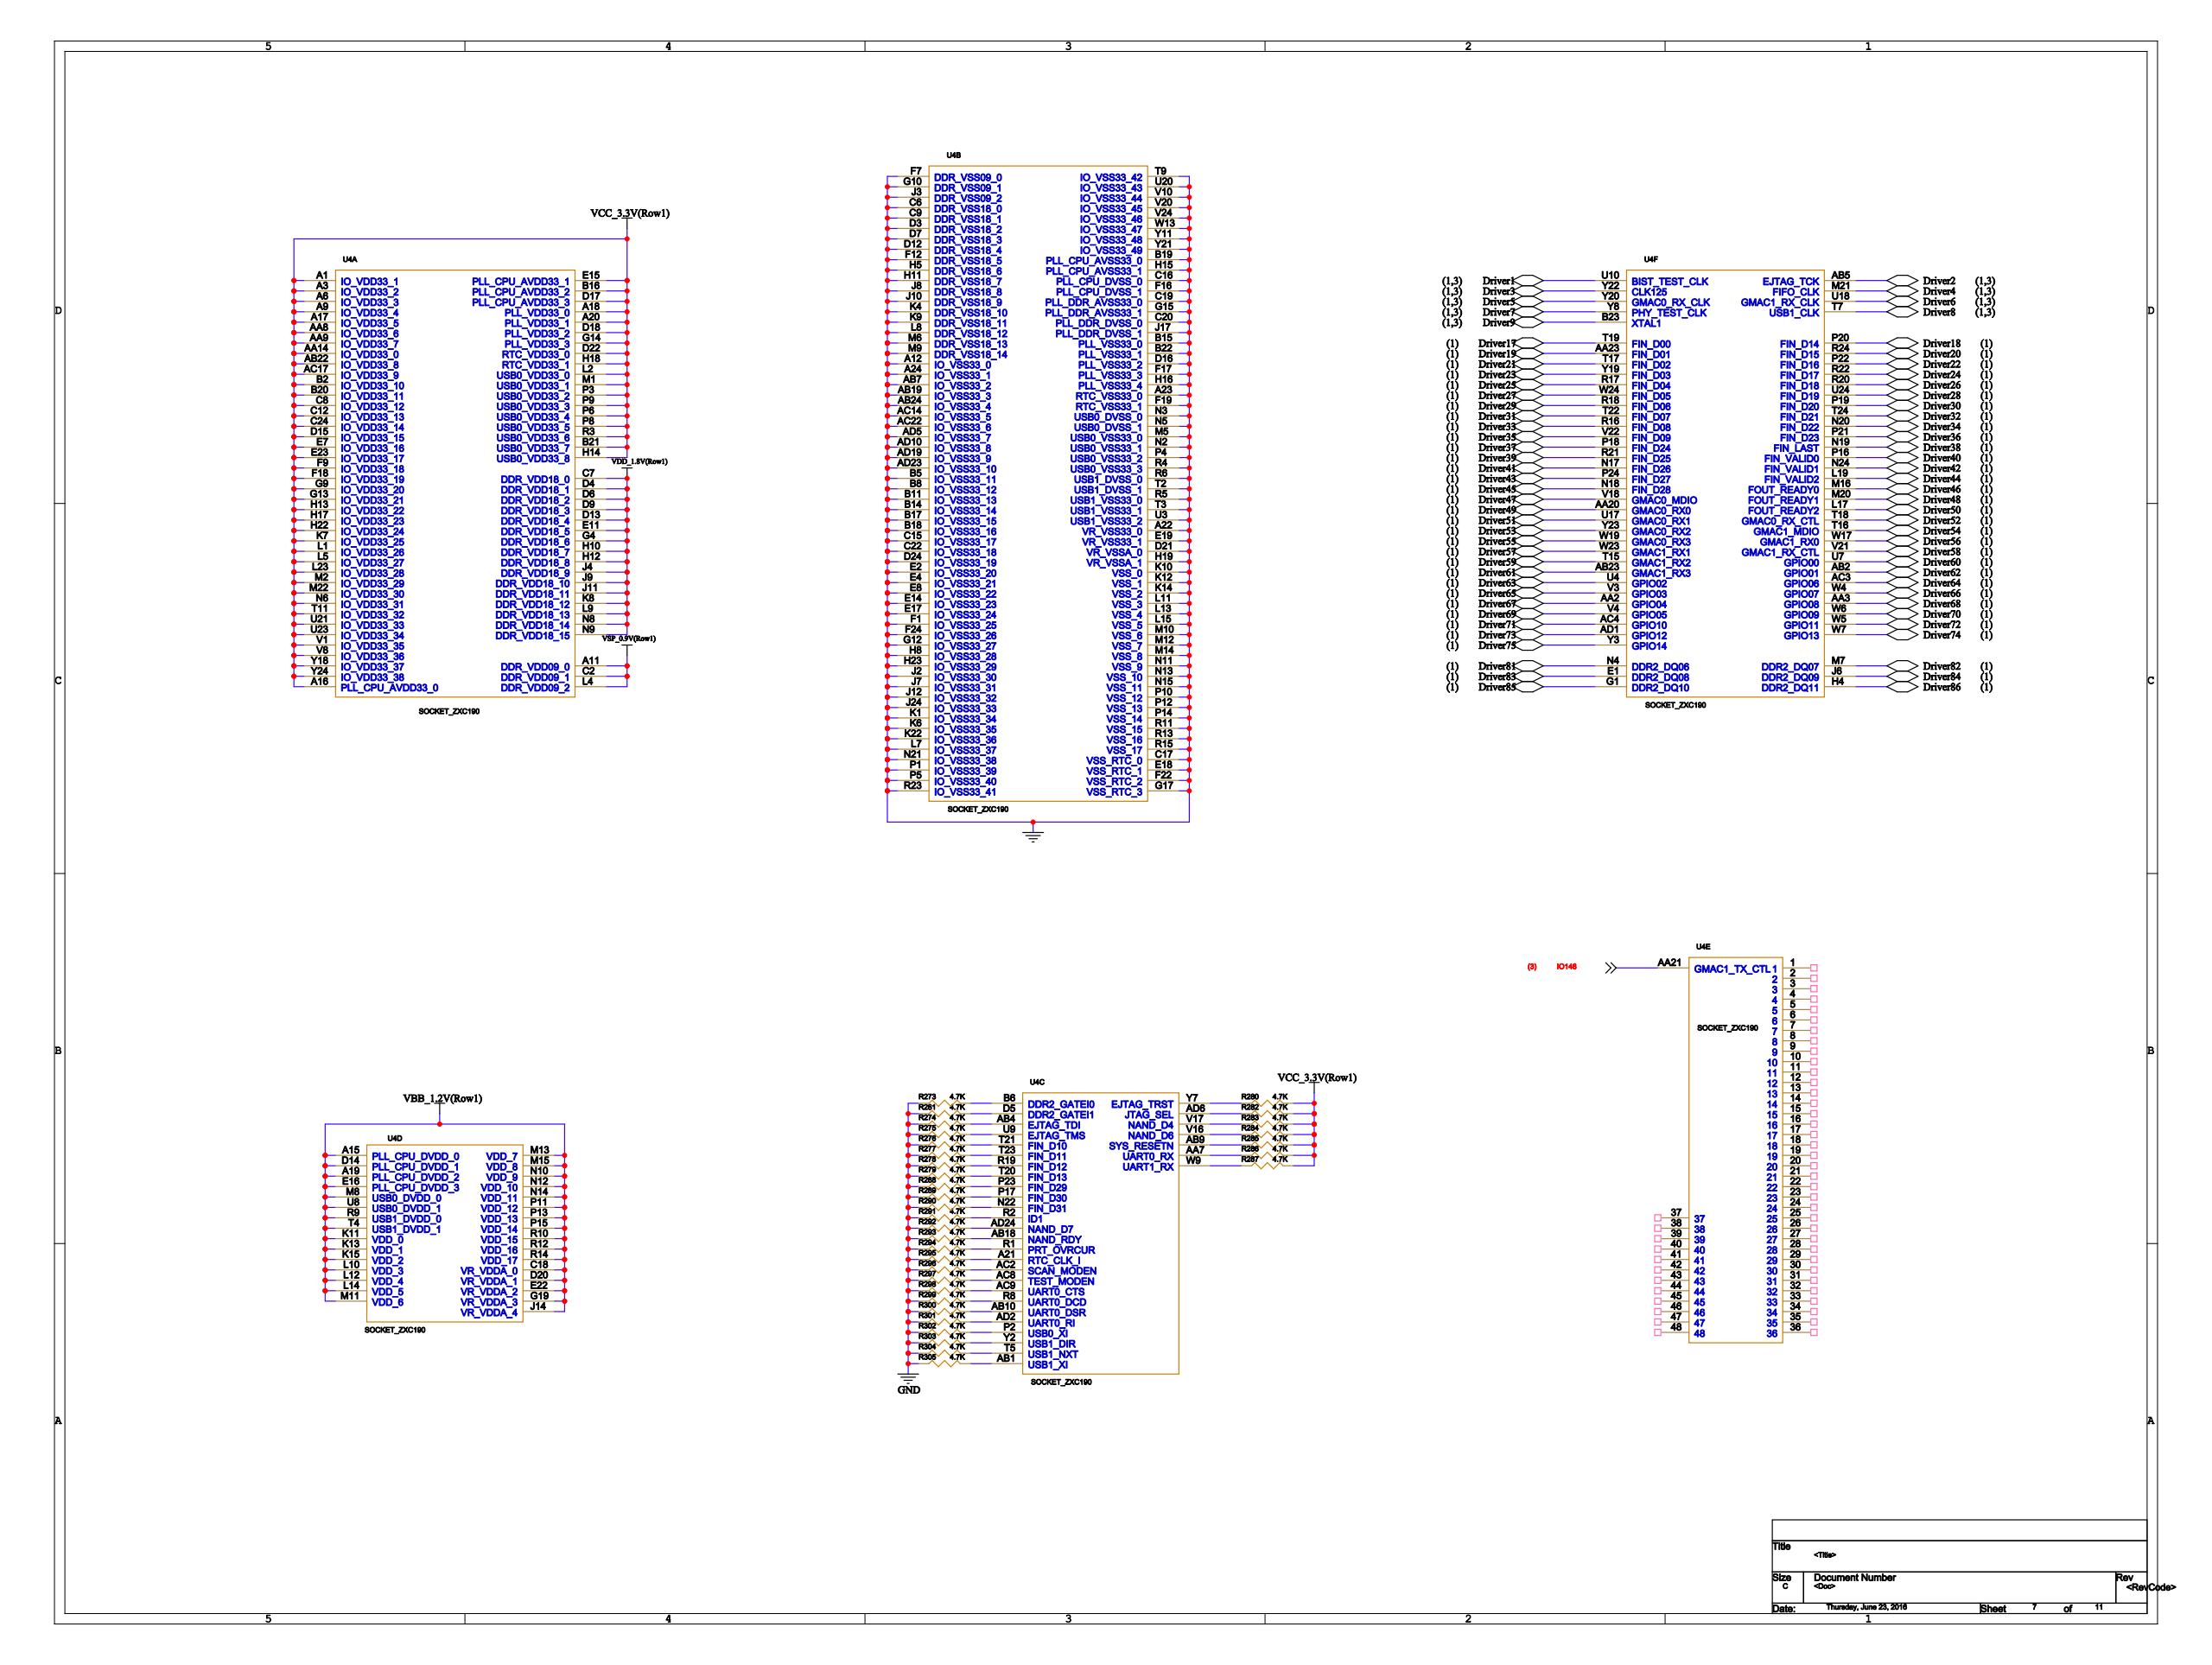Circuit board | Cadence Allegro | 531 parts | 624 nets | one sheet of the schematic
Parts on this sheet (reference | value | footprint):
R273 | 4.7K | R0805
R274 | 4.7K | R0805
R275 | 4.7K | R0805
R276 | 4.7K | R0805
R277 | 4.7K | R0805
R278 | 4.7K | R0805
R279 | 4.7K | R0805
R280 | 4.7K | R0805
R281 | 4.7K | R0805
R282 | 4.7K | R0805
R283 | 4.7K | R0805
R284 | 4.7K | R0805
R285 | 4.7K | R0805
R286 | 4.7K | R0805
R287 | 4.7K | R0805
R288 | 4.7K | R0805
R289 | 4.7K | R0805
R290 | 4.7K | R0805
R291 | 4.7K | R0805
R292 | 4.7K | R0805
R293 | 4.7K | R0805
R294 | 4.7K | R0805
R295 | 4.7K | R0805
R296 | 4.7K | R0805
R297 | 4.7K | R0805
R298 | 4.7K | R0805
R299 | 4.7K | R0805
R300 | 4.7K | R0805
R301 | 4.7K | R0805
R302 | 4.7K | R0805
R303 | 4.7K | R0805
R304 | 4.7K | R0805
R305 | 4.7K | R0805
U3 | SOCKET_ZXC190 | BGA-576
U4 | SOCKET_ZXC190 | BGA-576
U10 | SOCKET_ZXC190 | BGA-576
Nets of these parts (net: part-pin ...):
GND: R273-1 R274-1 R275-1 R276-1 R277-1 R278-1 R279-1 R281-1 R288-1 R289-1 R290-1 R291-1 R292-1 R293-1 R294-1 R295-1 R296-1 R297-1 R298-1 R299-1 R300-1 R301-1 R302-1 R303-1 R304-1 R305-1 U3-A12 U3-A22 U3-A23 U3-A24 U3-AB7 U3-AB19 U3-AB24 U3-AC14 U3-AC22 U3-AD5 U3-AD10 U3-AD19 U3-AD23 U3-B5 U3-B8 U3-B11 U3-B14 U3-B15 U3-B17 U3-B18 U3-B19 U3-B22 U3-C6 U3-C9 U3-C15 U3-C16 U3-C17 U3-C19 U3-C20 U3-C22 U3-D3 U3-D7 U3-D12 U3-D16 U3-D21 U3-D24 U3-E2 U3-E4 U3-E8 U3-E14 U3-E17 U3-E18 U3-E19 U3-F1 U3-F7 U3-F12 U3-F16 U3-F17 U3-F19 U3-F22 U3-F24 U3-G10 U3-G12 U3-G15 U3-G17 U3-H5 U3-H8 U3-H11 U3-H15 U3-H16 U3-H19 U3-H23 U3-J2 U3-J3 U3-J7 U3-J8 U3-J10 U3-J12 U3-J17 U3-J24 U3-K1 U3-K4 U3-K6 U3-K9 U3-K10 U3-K12 U3-K14 U3-K22 U3-L7 U3-L8 U3-L11 U3-L13 U3-L15 U3-M5 U3-M6 U3-M9 U3-M10 U3-M12 U3-M14 U3-N2 U3-N3 U3-N5 U3-N11 U3-N13 U3-N15 U3-N21 U3-P1 U3-P4 U3-P5 U3-P10 U3-P12 U3-P14 U3-R4 U3-R5 U3-R6 U3-R11 U3-R13 U3-R15 U3-R23 U3-T2 U3-T3 U3-T9 U3-U3 U3-U20 U3-V10 U3-V20 U3-V24 U3-W13 U3-Y11 U3-Y21 U4-A12 U4-A22 U4-A23 U4-A24 U4-AB7 U4-AB19 U4-AB24 U4-AC14 U4-AC22 U4-AD5 U4-AD10 U4-AD19 U4-AD23 U4-B5 U4-B8 U4-B11 U4-B14 U4-B15 U4-B17 U4-B18 U4-B19 U4-B22 U4-C6 U4-C9 U4-C15 U4-C16 U4-C17 U4-C19 U4-C20 U4-C22 U4-D3 U4-D7 U4-D12 U4-D16 U4-D21 U4-D24 U4-E2 U4-E4 U4-E8 U4-E14 U4-E17 U4-E18 U4-E19 U4-F1 U4-F7 U4-F12 U4-F16 U4-F17 U4-F19 U4-F22 U4-F24 U4-G10 U4-G12 U4-G15 U4-G17 U4-H5 U4-H8 U4-H11 U4-H15 U4-H16 U4-H19 U4-H23 U4-J2 U4-J3 U4-J7 U4-J8 U4-J10 U4-J12 U4-J17 U4-J24 U4-K1 U4-K4 U4-K6 U4-K9 U4-K10 U4-K12 U4-K14 U4-K22 U4-L7 U4-L8 U4-L11 U4-L13 U4-L15 U4-M5 U4-M6 U4-M9 U4-M10 U4-M12 U4-M14 U4-N2 U4-N3 U4-N5 U4-N11 U4-N13 U4-N15 U4-N21 U4-P1 U4-P4 U4-P5 U4-P10 U4-P12 U4-P14 U4-R4 U4-R5 U4-R6 U4-R11 U4-R13 U4-R15 U4-R23 U4-T2 U4-T3 U4-T9 U4-U3 U4-U20 U4-V10 U4-V20 U4-V24 U4-W13 U4-Y11 U4-Y21 U10-A12 U10-A22 U10-A23 U10-A24 U10-AB7 U10-AB19 U10-AB24 U10-AC14 U10-AC22 U10-AD5 U10-AD10 U10-AD19 U10-AD23 U10-B5 U10-B8 U10-B11 U10-B14 U10-B15 U10-B17 U10-B18 U10-B19 U10-B22 U10-C6 U10-C9 U10-C15 U10-C16 U10-C17 U10-C19 U10-C20 U10-C22 U10-D3 U10-D7 U10-D12 U10-D16 U10-D21 U10-D24 U10-E2 U10-E4 U10-E8 U10-E14 U10-E17 U10-E18 U10-E19 U10-F1 U10-F7 U10-F12 U10-F16 U10-F17 U10-F19 U10-F22 U10-F24 U10-G10 U10-G12 U10-G15 U10-G17 U10-H5 U10-H8 U10-H11 U10-H15 U10-H16 U10-H19 U10-H23 U10-J2 U10-J3 U10-J7 U10-J8 U10-J10 U10-J12 U10-J17 U10-J24 U10-K1 U10-K4 U10-K6 U10-K9 U10-K10 U10-K12 U10-K14 U10-K22 U10-L7 U10-L8 U10-L11 U10-L13 U10-L15 U10-M5 U10-M6 U10-M9 U10-M10 U10-M12 U10-M14 U10-N2 U10-N3 U10-N5 U10-N11 U10-N13 U10-N15 U10-N21 U10-P1 U10-P4 U10-P5 U10-P10 U10-P12 U10-P14 U10-R4 U10-R5 U10-R6 U10-R11 U10-R13 U10-R15 U10-R23 U10-T2 U10-T3 U10-T9 U10-U3 U10-U20 U10-V10 U10-V20 U10-V24 U10-W13 U10-Y11 U10-Y21
VCC_3.3V(ROW1): R280-2 R282-2 R283-2 R284-2 R285-2 R286-2 R287-2 U3-A1 U3-A3 U3-A6 U3-A9 U3-A16 U3-A17 U3-A18 U3-A20 U3-AA8 U3-AA9 U3-AA14 U3-AB22 U3-AC17 U3-B2 U3-B16 U3-B20 U3-B21 U3-C8 U3-C12 U3-C24 U3-D15 U3-D17 U3-D18 U3-D22 U3-E7 U3-E15 U3-E23 U3-F9 U3-F18 U3-G9 U3-G13 U3-G14 U3-H13 U3-H14 U3-H17 U3-H18 U3-H22 U3-K7 U3-L1 U3-L2 U3-L5 U3-L23 U3-M1 U3-M2 U3-M22 U3-N6 U3-P3 U3-P6 U3-P8 U3-P9 U3-R3 U3-T11 U3-U21 U3-U23 U3-V1 U3-V8 U3-Y18 U3-Y24 U4-A1 U4-A3 U4-A6 U4-A9 U4-A16 U4-A17 U4-A18 U4-A20 U4-AA8 U4-AA9 U4-AA14 U4-AB22 U4-AC17 U4-B2 U4-B16 U4-B20 U4-B21 U4-C8 U4-C12 U4-C24 U4-D15 U4-D17 U4-D18 U4-D22 U4-E7 U4-E15 U4-E23 U4-F9 U4-F18 U4-G9 U4-G13 U4-G14 U4-H13 U4-H14 U4-H17 U4-H18 U4-H22 U4-K7 U4-L1 U4-L2 U4-L5 U4-L23 U4-M1 U4-M2 U4-M22 U4-N6 U4-P3 U4-P6 U4-P8 U4-P9 U4-R3 U4-T11 U4-U21 U4-U23 U4-V1 U4-V8 U4-Y18 U4-Y24
N8549258: R273-2 U4-B6
N8549250: R274-2 U4-AB4
N8549246: R275-2 U4-U9
N8549242: R276-2 U4-T21
N8549238: R277-2 U4-T23
N8549234: R278-2 U4-R19
N8549290: R279-2 U4-T20
N8549682: R280-1 U4-Y7
N8549254: R281-2 U4-D5
N8549718: R282-1 U4-AD6
N8549862: R283-1 U4-V17
N8549866: R284-1 U4-V16
N8549890: R285-1 U4-AB9
N8549870: R286-1 U4-AA7
N8549214: R287-1 U4-W9
N8549286: R288-2 U4-P23
N8549282: R289-2 U4-P17
N8549278: R290-2 U4-N22
N8549274: R291-2 U4-R2
N8549270: R292-2 U4-AD24
N8549266: R293-2 U4-AB18
N8549262: R294-2 U4-R1
N8549318: R295-2 U4-A21
N8549314: R296-2 U4-AC2
N8549310: R297-2 U4-AC8
N8549306: R298-2 U4-AC9
N8549754: R299-2 U4-R8
N8549302: R300-2 U4-AB10
N8549298: R301-2 U4-AD2
N8549294: R302-2 U4-P2
N8549330: R303-2 U4-Y2
N8549326: R304-2 U4-T5
N8549322: R305-2 U4-AB1
IO148: U4-AA21